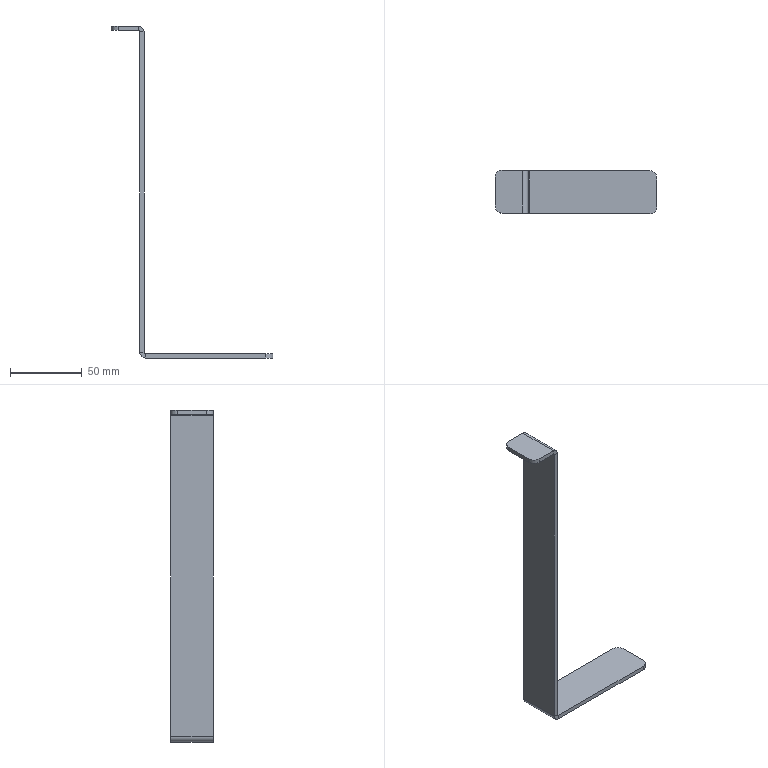Part | SolidWorks | features BreakCorner 1, FlatPattern 1, SMBaseFlange 1, SheetMetal 1 | 1 solid | 26 faces | box 113 x 30 x 232 mm | volume 30522 mm3 | plane 18 | cylinder 8 | commonest cylinder face diameters 10 x4 2 x2 8 x2
STEP:
#1=CARTESIAN_POINT('',(20.,15.,-1.));
#2=VERTEX_POINT('',#1);
#3=CARTESIAN_POINT('',(23.,15.,-1.));
#4=VERTEX_POINT('',#3);
#5=CARTESIAN_POINT('',(20.,15.,-1.));
#6=DIRECTION('',(1.,0.,0.));
#7=VECTOR('',#6,1000.);
#8=LINE('',#5,#7);
#9=EDGE_CURVE('',#2,#4,#8,.T.);
#10=ORIENTED_EDGE('',*,*,#9,.F.);
#11=CARTESIAN_POINT('',(19.,15.,0.));
#12=VERTEX_POINT('',#11);
#13=CARTESIAN_POINT('',(19.,15.,-1.));
#14=DIRECTION('',(0.,1.,0.));
#15=DIRECTION('',(0.,0.,-1.));
#16=AXIS2_PLACEMENT_3D('',#13,#14,#15);
#17=CIRCLE('',#16,1.);
#18=EDGE_CURVE('',#12,#2,#17,.T.);
#19=ORIENTED_EDGE('',*,*,#18,.F.);
#20=CARTESIAN_POINT('',(19.,15.,3.));
#21=VERTEX_POINT('',#20);
#22=CARTESIAN_POINT('',(19.,15.,3.));
#23=DIRECTION('',(0.,0.,-1.));
#24=VECTOR('',#23,1000.);
#25=LINE('',#22,#24);
#26=EDGE_CURVE('',#21,#12,#25,.T.);
#27=ORIENTED_EDGE('',*,*,#26,.F.);
#28=CARTESIAN_POINT('',(19.,15.,-1.));
#29=DIRECTION('',(0.,1.,0.));
#30=DIRECTION('',(1.,0.,0.));
#31=AXIS2_PLACEMENT_3D('',#28,#29,#30);
#32=CIRCLE('',#31,4.);
#33=EDGE_CURVE('',#21,#4,#32,.T.);
#34=ORIENTED_EDGE('',*,*,#33,.T.);
#35=EDGE_LOOP('',(#10,#19,#27,#34));
#36=FACE_OUTER_BOUND('',#35,.T.);
#37=CARTESIAN_POINT('',(20.,15.,-1.));
#38=DIRECTION('',(0.,1.,0.));
#39=DIRECTION('',(0.,0.,1.));
#40=AXIS2_PLACEMENT_3D('',#37,#38,#39);
#41=PLANE('',#40);
#42=ADVANCED_FACE('',(#36),#41,.T.);
#43=CARTESIAN_POINT('',(20.,15.,-225.));
#44=VERTEX_POINT('',#43);
#45=CARTESIAN_POINT('',(20.,15.,0.));
#46=DIRECTION('',(0.,0.,-1.));
#47=VECTOR('',#46,1000.);
#48=LINE('',#45,#47);
#49=EDGE_CURVE('',#2,#44,#48,.T.);
#50=ORIENTED_EDGE('',*,*,#49,.F.);
#51=ORIENTED_EDGE('',*,*,#9,.T.);
#52=CARTESIAN_POINT('',(23.,15.,-225.));
#53=VERTEX_POINT('',#52);
#54=CARTESIAN_POINT('',(23.,15.,0.));
#55=DIRECTION('',(0.,0.,-1.));
#56=VECTOR('',#55,1000.);
#57=LINE('',#54,#56);
#58=EDGE_CURVE('',#4,#53,#57,.T.);
#59=ORIENTED_EDGE('',*,*,#58,.T.);
#60=CARTESIAN_POINT('',(23.,15.,-225.));
#61=DIRECTION('',(-1.,0.,0.));
#62=VECTOR('',#61,1000.);
#63=LINE('',#60,#62);
#64=EDGE_CURVE('',#53,#44,#63,.T.);
#65=ORIENTED_EDGE('',*,*,#64,.T.);
#66=EDGE_LOOP('',(#50,#51,#59,#65));
#67=FACE_OUTER_BOUND('',#66,.T.);
#68=CARTESIAN_POINT('',(19.,15.,3.));
#69=DIRECTION('',(0.,1.,0.));
#70=DIRECTION('',(0.,0.,1.));
#71=AXIS2_PLACEMENT_3D('',#68,#69,#70);
#72=PLANE('',#71);
#73=ADVANCED_FACE('',(#67),#72,.T.);
#74=CARTESIAN_POINT('',(19.,-15.,0.));
#75=VERTEX_POINT('',#74);
#76=CARTESIAN_POINT('',(19.,-15.,3.));
#77=VERTEX_POINT('',#76);
#78=CARTESIAN_POINT('',(19.,-15.,0.));
#79=DIRECTION('',(0.,0.,1.));
#80=VECTOR('',#79,1000.);
#81=LINE('',#78,#80);
#82=EDGE_CURVE('',#75,#77,#81,.T.);
#83=ORIENTED_EDGE('',*,*,#82,.F.);
#84=CARTESIAN_POINT('',(20.,-15.,-1.));
#85=VERTEX_POINT('',#84);
#86=CARTESIAN_POINT('',(19.,-15.,-1.));
#87=DIRECTION('',(0.,1.,0.));
#88=DIRECTION('',(0.,0.,-1.));
#89=AXIS2_PLACEMENT_3D('',#86,#87,#88);
#90=CIRCLE('',#89,1.);
#91=EDGE_CURVE('',#75,#85,#90,.T.);
#92=ORIENTED_EDGE('',*,*,#91,.T.);
#93=CARTESIAN_POINT('',(23.,-15.,-1.));
#94=VERTEX_POINT('',#93);
#95=CARTESIAN_POINT('',(23.,-15.,-1.));
#96=DIRECTION('',(-1.,0.,0.));
#97=VECTOR('',#96,1000.);
#98=LINE('',#95,#97);
#99=EDGE_CURVE('',#94,#85,#98,.T.);
#100=ORIENTED_EDGE('',*,*,#99,.F.);
#101=CARTESIAN_POINT('',(19.,-15.,-1.));
#102=DIRECTION('',(0.,1.,0.));
#103=DIRECTION('',(1.,0.,0.));
#104=AXIS2_PLACEMENT_3D('',#101,#102,#103);
#105=CIRCLE('',#104,4.);
#106=EDGE_CURVE('',#77,#94,#105,.T.);
#107=ORIENTED_EDGE('',*,*,#106,.F.);
#108=EDGE_LOOP('',(#83,#92,#100,#107));
#109=FACE_OUTER_BOUND('',#108,.T.);
#110=CARTESIAN_POINT('',(19.,-15.,0.));
#111=DIRECTION('',(0.,-1.,0.));
#112=DIRECTION('',(0.,0.,-1.));
#113=AXIS2_PLACEMENT_3D('',#110,#111,#112);
#114=PLANE('',#113);
#115=ADVANCED_FACE('',(#109),#114,.T.);
#116=CARTESIAN_POINT('',(5.,-15.,3.));
#117=VERTEX_POINT('',#116);
#118=CARTESIAN_POINT('',(0.,-15.,3.));
#119=DIRECTION('',(1.,0.,0.));
#120=VECTOR('',#119,1000.);
#121=LINE('',#118,#120);
#122=EDGE_CURVE('',#117,#77,#121,.T.);
#123=ORIENTED_EDGE('',*,*,#122,.F.);
#124=CARTESIAN_POINT('',(5.,-15.,0.));
#125=VERTEX_POINT('',#124);
#126=CARTESIAN_POINT('',(5.,-15.,-1.));
#127=DIRECTION('',(0.,0.,-1.));
#128=VECTOR('',#127,1000.);
#129=LINE('',#126,#128);
#130=EDGE_CURVE('',#117,#125,#129,.T.);
#131=ORIENTED_EDGE('',*,*,#130,.T.);
#132=CARTESIAN_POINT('',(0.,-15.,0.));
#133=DIRECTION('',(1.,0.,0.));
#134=VECTOR('',#133,1000.);
#135=LINE('',#132,#134);
#136=EDGE_CURVE('',#125,#75,#135,.T.);
#137=ORIENTED_EDGE('',*,*,#136,.T.);
#138=ORIENTED_EDGE('',*,*,#82,.T.);
#139=EDGE_LOOP('',(#123,#131,#137,#138));
#140=FACE_OUTER_BOUND('',#139,.T.);
#141=CARTESIAN_POINT('',(23.,-15.,-1.));
#142=DIRECTION('',(0.,-1.,0.));
#143=DIRECTION('',(0.,0.,-1.));
#144=AXIS2_PLACEMENT_3D('',#141,#142,#143);
#145=PLANE('',#144);
#146=ADVANCED_FACE('',(#140),#145,.T.);
#147=CARTESIAN_POINT('',(24.,15.,-229.));
#148=VERTEX_POINT('',#147);
#149=CARTESIAN_POINT('',(24.,15.,-226.));
#150=VERTEX_POINT('',#149);
#151=CARTESIAN_POINT('',(24.,15.,-229.));
#152=DIRECTION('',(0.,0.,1.));
#153=VECTOR('',#152,1000.);
#154=LINE('',#151,#153);
#155=EDGE_CURVE('',#148,#150,#154,.T.);
#156=ORIENTED_EDGE('',*,*,#155,.F.);
#157=CARTESIAN_POINT('',(24.,15.,-225.));
#158=DIRECTION('',(0.,-1.,0.));
#159=DIRECTION('',(0.,0.,1.));
#160=AXIS2_PLACEMENT_3D('',#157,#158,#159);
#161=CIRCLE('',#160,4.);
#162=EDGE_CURVE('',#44,#148,#161,.T.);
#163=ORIENTED_EDGE('',*,*,#162,.F.);
#164=ORIENTED_EDGE('',*,*,#64,.F.);
#165=CARTESIAN_POINT('',(24.,15.,-225.));
#166=DIRECTION('',(0.,-1.,0.));
#167=DIRECTION('',(1.,0.,0.));
#168=AXIS2_PLACEMENT_3D('',#165,#166,#167);
#169=CIRCLE('',#168,1.);
#170=EDGE_CURVE('',#53,#150,#169,.T.);
#171=ORIENTED_EDGE('',*,*,#170,.T.);
#172=EDGE_LOOP('',(#156,#163,#164,#171));
#173=FACE_OUTER_BOUND('',#172,.T.);
#174=CARTESIAN_POINT('',(24.,15.,-229.));
#175=DIRECTION('',(0.,1.,0.));
#176=DIRECTION('',(0.,0.,1.));
#177=AXIS2_PLACEMENT_3D('',#174,#175,#176);
#178=PLANE('',#177);
#179=ADVANCED_FACE('',(#173),#178,.T.);
#180=CARTESIAN_POINT('',(108.,15.,-226.));
#181=VERTEX_POINT('',#180);
#182=CARTESIAN_POINT('',(20.,15.,-226.));
#183=DIRECTION('',(1.,0.,0.));
#184=VECTOR('',#183,1000.);
#185=LINE('',#182,#184);
#186=EDGE_CURVE('',#150,#181,#185,.T.);
#187=ORIENTED_EDGE('',*,*,#186,.T.);
#188=CARTESIAN_POINT('',(108.,15.,-229.));
#189=VERTEX_POINT('',#188);
#190=CARTESIAN_POINT('',(108.,15.,-225.));
#191=DIRECTION('',(0.,0.,-1.));
#192=VECTOR('',#191,1000.);
#193=LINE('',#190,#192);
#194=EDGE_CURVE('',#181,#189,#193,.T.);
#195=ORIENTED_EDGE('',*,*,#194,.T.);
#196=CARTESIAN_POINT('',(20.,15.,-229.));
#197=DIRECTION('',(1.,0.,0.));
#198=VECTOR('',#197,1000.);
#199=LINE('',#196,#198);
#200=EDGE_CURVE('',#148,#189,#199,.T.);
#201=ORIENTED_EDGE('',*,*,#200,.F.);
#202=ORIENTED_EDGE('',*,*,#155,.T.);
#203=EDGE_LOOP('',(#187,#195,#201,#202));
#204=FACE_OUTER_BOUND('',#203,.T.);
#205=CARTESIAN_POINT('',(23.,15.,-225.));
#206=DIRECTION('',(0.,1.,0.));
#207=DIRECTION('',(0.,0.,1.));
#208=AXIS2_PLACEMENT_3D('',#205,#206,#207);
#209=PLANE('',#208);
#210=ADVANCED_FACE('',(#204),#209,.T.);
#211=CARTESIAN_POINT('',(20.,-15.,-225.));
#212=VERTEX_POINT('',#211);
#213=CARTESIAN_POINT('',(23.,-15.,-225.));
#214=VERTEX_POINT('',#213);
#215=CARTESIAN_POINT('',(20.,-15.,-225.));
#216=DIRECTION('',(1.,0.,0.));
#217=VECTOR('',#216,1000.);
#218=LINE('',#215,#217);
#219=EDGE_CURVE('',#212,#214,#218,.T.);
#220=ORIENTED_EDGE('',*,*,#219,.F.);
#221=CARTESIAN_POINT('',(24.,-15.,-229.));
#222=VERTEX_POINT('',#221);
#223=CARTESIAN_POINT('',(24.,-15.,-225.));
#224=DIRECTION('',(0.,-1.,0.));
#225=DIRECTION('',(0.,0.,1.));
#226=AXIS2_PLACEMENT_3D('',#223,#224,#225);
#227=CIRCLE('',#226,4.);
#228=EDGE_CURVE('',#212,#222,#227,.T.);
#229=ORIENTED_EDGE('',*,*,#228,.T.);
#230=CARTESIAN_POINT('',(24.,-15.,-226.));
#231=VERTEX_POINT('',#230);
#232=CARTESIAN_POINT('',(24.,-15.,-226.));
#233=DIRECTION('',(0.,0.,-1.));
#234=VECTOR('',#233,1000.);
#235=LINE('',#232,#234);
#236=EDGE_CURVE('',#231,#222,#235,.T.);
#237=ORIENTED_EDGE('',*,*,#236,.F.);
#238=CARTESIAN_POINT('',(24.,-15.,-225.));
#239=DIRECTION('',(0.,-1.,0.));
#240=DIRECTION('',(1.,0.,0.));
#241=AXIS2_PLACEMENT_3D('',#238,#239,#240);
#242=CIRCLE('',#241,1.);
#243=EDGE_CURVE('',#214,#231,#242,.T.);
#244=ORIENTED_EDGE('',*,*,#243,.F.);
#245=EDGE_LOOP('',(#220,#229,#237,#244));
#246=FACE_OUTER_BOUND('',#245,.T.);
#247=CARTESIAN_POINT('',(20.,-15.,-225.));
#248=DIRECTION('',(0.,-1.,0.));
#249=DIRECTION('',(0.,0.,-1.));
#250=AXIS2_PLACEMENT_3D('',#247,#248,#249);
#251=PLANE('',#250);
#252=ADVANCED_FACE('',(#246),#251,.T.);
#253=CARTESIAN_POINT('',(20.,-15.,0.));
#254=DIRECTION('',(0.,0.,-1.));
#255=VECTOR('',#254,1000.);
#256=LINE('',#253,#255);
#257=EDGE_CURVE('',#85,#212,#256,.T.);
#258=ORIENTED_EDGE('',*,*,#257,.T.);
#259=ORIENTED_EDGE('',*,*,#219,.T.);
#260=CARTESIAN_POINT('',(23.,-15.,0.));
#261=DIRECTION('',(0.,0.,-1.));
#262=VECTOR('',#261,1000.);
#263=LINE('',#260,#262);
#264=EDGE_CURVE('',#94,#214,#263,.T.);
#265=ORIENTED_EDGE('',*,*,#264,.F.);
#266=ORIENTED_EDGE('',*,*,#99,.T.);
#267=EDGE_LOOP('',(#258,#259,#265,#266));
#268=FACE_OUTER_BOUND('',#267,.T.);
#269=CARTESIAN_POINT('',(24.,-15.,-226.));
#270=DIRECTION('',(0.,-1.,0.));
#271=DIRECTION('',(0.,0.,-1.));
#272=AXIS2_PLACEMENT_3D('',#269,#270,#271);
#273=PLANE('',#272);
#274=ADVANCED_FACE('',(#268),#273,.T.);
#275=CARTESIAN_POINT('',(113.,10.,-226.));
#276=VERTEX_POINT('',#275);
#277=CARTESIAN_POINT('',(113.,-10.,-226.));
#278=VERTEX_POINT('',#277);
#279=CARTESIAN_POINT('',(113.,15.,-226.));
#280=DIRECTION('',(0.,-1.,0.));
#281=VECTOR('',#280,1000.);
#282=LINE('',#279,#281);
#283=EDGE_CURVE('',#276,#278,#282,.T.);
#284=ORIENTED_EDGE('',*,*,#283,.F.);
#285=CARTESIAN_POINT('',(108.,10.,-226.));
#286=DIRECTION('',(0.,0.,1.));
#287=DIRECTION('',(-1.,0.,0.));
#288=AXIS2_PLACEMENT_3D('',#285,#286,#287);
#289=CIRCLE('',#288,5.);
#290=EDGE_CURVE('',#276,#181,#289,.T.);
#291=ORIENTED_EDGE('',*,*,#290,.T.);
#292=ORIENTED_EDGE('',*,*,#186,.F.);
#293=CARTESIAN_POINT('',(24.,15.,-226.));
#294=DIRECTION('',(0.,-1.,0.));
#295=VECTOR('',#294,1000.);
#296=LINE('',#293,#295);
#297=EDGE_CURVE('',#150,#231,#296,.T.);
#298=ORIENTED_EDGE('',*,*,#297,.T.);
#299=CARTESIAN_POINT('',(108.,-15.,-226.));
#300=VERTEX_POINT('',#299);
#301=CARTESIAN_POINT('',(20.,-15.,-226.));
#302=DIRECTION('',(1.,0.,0.));
#303=VECTOR('',#302,1000.);
#304=LINE('',#301,#303);
#305=EDGE_CURVE('',#231,#300,#304,.T.);
#306=ORIENTED_EDGE('',*,*,#305,.T.);
#307=CARTESIAN_POINT('',(108.,-10.,-226.));
#308=DIRECTION('',(0.,0.,1.));
#309=DIRECTION('',(-1.,0.,0.));
#310=AXIS2_PLACEMENT_3D('',#307,#308,#309);
#311=CIRCLE('',#310,5.);
#312=EDGE_CURVE('',#300,#278,#311,.T.);
#313=ORIENTED_EDGE('',*,*,#312,.T.);
#314=EDGE_LOOP('',(#284,#291,#292,#298,#306,#313));
#315=FACE_OUTER_BOUND('',#314,.T.);
#316=CARTESIAN_POINT('',(20.,15.,-226.));
#317=DIRECTION('',(0.,0.,-1.));
#318=DIRECTION('',(-1.,0.,0.));
#319=AXIS2_PLACEMENT_3D('',#316,#317,#318);
#320=PLANE('',#319);
#321=ADVANCED_FACE('',(#315),#320,.F.);
#322=CARTESIAN_POINT('',(113.,10.,-229.));
#323=VERTEX_POINT('',#322);
#324=CARTESIAN_POINT('',(113.,-10.,-229.));
#325=VERTEX_POINT('',#324);
#326=CARTESIAN_POINT('',(113.,15.,-229.));
#327=DIRECTION('',(0.,-1.,0.));
#328=VECTOR('',#327,1000.);
#329=LINE('',#326,#328);
#330=EDGE_CURVE('',#323,#325,#329,.T.);
#331=ORIENTED_EDGE('',*,*,#330,.F.);
#332=CARTESIAN_POINT('',(113.,10.,-229.));
#333=DIRECTION('',(0.,0.,1.));
#334=VECTOR('',#333,1000.);
#335=LINE('',#332,#334);
#336=EDGE_CURVE('',#323,#276,#335,.T.);
#337=ORIENTED_EDGE('',*,*,#336,.T.);
#338=ORIENTED_EDGE('',*,*,#283,.T.);
#339=CARTESIAN_POINT('',(113.,-10.,-229.));
#340=DIRECTION('',(0.,0.,-1.));
#341=VECTOR('',#340,1000.);
#342=LINE('',#339,#341);
#343=EDGE_CURVE('',#278,#325,#342,.T.);
#344=ORIENTED_EDGE('',*,*,#343,.T.);
#345=EDGE_LOOP('',(#331,#337,#338,#344));
#346=FACE_OUTER_BOUND('',#345,.T.);
#347=CARTESIAN_POINT('',(113.,15.,-229.));
#348=DIRECTION('',(1.,0.,0.));
#349=DIRECTION('',(0.,0.,-1.));
#350=AXIS2_PLACEMENT_3D('',#347,#348,#349);
#351=PLANE('',#350);
#352=ADVANCED_FACE('',(#346),#351,.T.);
#353=ORIENTED_EDGE('',*,*,#200,.T.);
#354=CARTESIAN_POINT('',(108.,10.,-229.));
#355=DIRECTION('',(0.,0.,-1.));
#356=DIRECTION('',(-1.,0.,0.));
#357=AXIS2_PLACEMENT_3D('',#354,#355,#356);
#358=CIRCLE('',#357,5.);
#359=EDGE_CURVE('',#189,#323,#358,.T.);
#360=ORIENTED_EDGE('',*,*,#359,.T.);
#361=ORIENTED_EDGE('',*,*,#330,.T.);
#362=CARTESIAN_POINT('',(108.,-15.,-229.));
#363=VERTEX_POINT('',#362);
#364=CARTESIAN_POINT('',(108.,-10.,-229.));
#365=DIRECTION('',(0.,0.,-1.));
#366=DIRECTION('',(-1.,0.,0.));
#367=AXIS2_PLACEMENT_3D('',#364,#365,#366);
#368=CIRCLE('',#367,5.);
#369=EDGE_CURVE('',#325,#363,#368,.T.);
#370=ORIENTED_EDGE('',*,*,#369,.T.);
#371=CARTESIAN_POINT('',(20.,-15.,-229.));
#372=DIRECTION('',(1.,0.,0.));
#373=VECTOR('',#372,1000.);
#374=LINE('',#371,#373);
#375=EDGE_CURVE('',#222,#363,#374,.T.);
#376=ORIENTED_EDGE('',*,*,#375,.F.);
#377=CARTESIAN_POINT('',(24.,15.,-229.));
#378=DIRECTION('',(0.,-1.,0.));
#379=VECTOR('',#378,1000.);
#380=LINE('',#377,#379);
#381=EDGE_CURVE('',#148,#222,#380,.T.);
#382=ORIENTED_EDGE('',*,*,#381,.F.);
#383=EDGE_LOOP('',(#353,#360,#361,#370,#376,#382));
#384=FACE_OUTER_BOUND('',#383,.T.);
#385=CARTESIAN_POINT('',(20.,15.,-229.));
#386=DIRECTION('',(0.,0.,-1.));
#387=DIRECTION('',(-1.,0.,0.));
#388=AXIS2_PLACEMENT_3D('',#385,#386,#387);
#389=PLANE('',#388);
#390=ADVANCED_FACE('',(#384),#389,.T.);
#391=ORIENTED_EDGE('',*,*,#228,.F.);
#392=CARTESIAN_POINT('',(20.,15.,-225.));
#393=DIRECTION('',(0.,-1.,0.));
#394=VECTOR('',#393,1000.);
#395=LINE('',#392,#394);
#396=EDGE_CURVE('',#44,#212,#395,.T.);
#397=ORIENTED_EDGE('',*,*,#396,.F.);
#398=ORIENTED_EDGE('',*,*,#162,.T.);
#399=ORIENTED_EDGE('',*,*,#381,.T.);
#400=EDGE_LOOP('',(#391,#397,#398,#399));
#401=FACE_OUTER_BOUND('',#400,.T.);
#402=CARTESIAN_POINT('',(24.,15.,-225.));
#403=DIRECTION('',(0.,-1.,0.));
#404=DIRECTION('',(0.,0.,-1.));
#405=AXIS2_PLACEMENT_3D('',#402,#403,#404);
#406=CYLINDRICAL_SURFACE('',#405,4.);
#407=ADVANCED_FACE('',(#401),#406,.T.);
#408=ORIENTED_EDGE('',*,*,#257,.F.);
#409=CARTESIAN_POINT('',(20.,15.,-1.));
#410=DIRECTION('',(0.,-1.,0.));
#411=VECTOR('',#410,1000.);
#412=LINE('',#409,#411);
#413=EDGE_CURVE('',#2,#85,#412,.T.);
#414=ORIENTED_EDGE('',*,*,#413,.F.);
#415=ORIENTED_EDGE('',*,*,#49,.T.);
#416=ORIENTED_EDGE('',*,*,#396,.T.);
#417=EDGE_LOOP('',(#408,#414,#415,#416));
#418=FACE_OUTER_BOUND('',#417,.T.);
#419=CARTESIAN_POINT('',(20.,15.,0.));
#420=DIRECTION('',(-1.,0.,0.));
#421=DIRECTION('',(0.,0.,1.));
#422=AXIS2_PLACEMENT_3D('',#419,#420,#421);
#423=PLANE('',#422);
#424=ADVANCED_FACE('',(#418),#423,.T.);
#425=ORIENTED_EDGE('',*,*,#91,.F.);
#426=CARTESIAN_POINT('',(19.,15.,0.));
#427=DIRECTION('',(0.,-1.,0.));
#428=VECTOR('',#427,1000.);
#429=LINE('',#426,#428);
#430=EDGE_CURVE('',#12,#75,#429,.T.);
#431=ORIENTED_EDGE('',*,*,#430,.F.);
#432=ORIENTED_EDGE('',*,*,#18,.T.);
#433=ORIENTED_EDGE('',*,*,#413,.T.);
#434=EDGE_LOOP('',(#425,#431,#432,#433));
#435=FACE_OUTER_BOUND('',#434,.T.);
#436=CARTESIAN_POINT('',(19.,15.,-1.));
#437=DIRECTION('',(0.,-1.,0.));
#438=DIRECTION('',(0.,0.,-1.));
#439=AXIS2_PLACEMENT_3D('',#436,#437,#438);
#440=CYLINDRICAL_SURFACE('',#439,1.);
#441=ADVANCED_FACE('',(#435),#440,.F.);
#442=CARTESIAN_POINT('',(0.,10.,0.));
#443=VERTEX_POINT('',#442);
#444=CARTESIAN_POINT('',(0.,-10.,0.));
#445=VERTEX_POINT('',#444);
#446=CARTESIAN_POINT('',(0.,15.,0.));
#447=DIRECTION('',(0.,-1.,0.));
#448=VECTOR('',#447,1000.);
#449=LINE('',#446,#448);
#450=EDGE_CURVE('',#443,#445,#449,.T.);
#451=ORIENTED_EDGE('',*,*,#450,.F.);
#452=CARTESIAN_POINT('',(5.,15.,0.));
#453=VERTEX_POINT('',#452);
#454=CARTESIAN_POINT('',(5.,10.,0.));
#455=DIRECTION('',(0.,0.,-1.));
#456=DIRECTION('',(-1.,0.,0.));
#457=AXIS2_PLACEMENT_3D('',#454,#455,#456);
#458=CIRCLE('',#457,5.);
#459=EDGE_CURVE('',#443,#453,#458,.T.);
#460=ORIENTED_EDGE('',*,*,#459,.T.);
#461=CARTESIAN_POINT('',(0.,15.,0.));
#462=DIRECTION('',(1.,0.,0.));
#463=VECTOR('',#462,1000.);
#464=LINE('',#461,#463);
#465=EDGE_CURVE('',#453,#12,#464,.T.);
#466=ORIENTED_EDGE('',*,*,#465,.T.);
#467=ORIENTED_EDGE('',*,*,#430,.T.);
#468=ORIENTED_EDGE('',*,*,#136,.F.);
#469=CARTESIAN_POINT('',(5.,-10.,0.));
#470=DIRECTION('',(0.,0.,-1.));
#471=DIRECTION('',(-1.,0.,0.));
#472=AXIS2_PLACEMENT_3D('',#469,#470,#471);
#473=CIRCLE('',#472,5.);
#474=EDGE_CURVE('',#125,#445,#473,.T.);
#475=ORIENTED_EDGE('',*,*,#474,.T.);
#476=EDGE_LOOP('',(#451,#460,#466,#467,#468,#475));
#477=FACE_OUTER_BOUND('',#476,.T.);
#478=CARTESIAN_POINT('',(0.,15.,0.));
#479=DIRECTION('',(0.,0.,-1.));
#480=DIRECTION('',(-1.,0.,0.));
#481=AXIS2_PLACEMENT_3D('',#478,#479,#480);
#482=PLANE('',#481);
#483=ADVANCED_FACE('',(#477),#482,.T.);
#484=CARTESIAN_POINT('',(0.,10.,3.));
#485=VERTEX_POINT('',#484);
#486=CARTESIAN_POINT('',(0.,-10.,3.));
#487=VERTEX_POINT('',#486);
#488=CARTESIAN_POINT('',(0.,15.,3.));
#489=DIRECTION('',(0.,-1.,0.));
#490=VECTOR('',#489,1000.);
#491=LINE('',#488,#490);
#492=EDGE_CURVE('',#485,#487,#491,.T.);
#493=ORIENTED_EDGE('',*,*,#492,.F.);
#494=CARTESIAN_POINT('',(0.,10.,3.));
#495=DIRECTION('',(0.,0.,-1.));
#496=VECTOR('',#495,1000.);
#497=LINE('',#494,#496);
#498=EDGE_CURVE('',#485,#443,#497,.T.);
#499=ORIENTED_EDGE('',*,*,#498,.T.);
#500=ORIENTED_EDGE('',*,*,#450,.T.);
#501=CARTESIAN_POINT('',(0.,-10.,3.));
#502=DIRECTION('',(0.,0.,1.));
#503=VECTOR('',#502,1000.);
#504=LINE('',#501,#503);
#505=EDGE_CURVE('',#445,#487,#504,.T.);
#506=ORIENTED_EDGE('',*,*,#505,.T.);
#507=EDGE_LOOP('',(#493,#499,#500,#506));
#508=FACE_OUTER_BOUND('',#507,.T.);
#509=CARTESIAN_POINT('',(0.,15.,3.));
#510=DIRECTION('',(-1.,0.,0.));
#511=DIRECTION('',(0.,0.,1.));
#512=AXIS2_PLACEMENT_3D('',#509,#510,#511);
#513=PLANE('',#512);
#514=ADVANCED_FACE('',(#508),#513,.T.);
#515=CARTESIAN_POINT('',(5.,15.,3.));
#516=VERTEX_POINT('',#515);
#517=CARTESIAN_POINT('',(0.,15.,3.));
#518=DIRECTION('',(1.,0.,0.));
#519=VECTOR('',#518,1000.);
#520=LINE('',#517,#519);
#521=EDGE_CURVE('',#516,#21,#520,.T.);
#522=ORIENTED_EDGE('',*,*,#521,.F.);
#523=CARTESIAN_POINT('',(5.,10.,3.));
#524=DIRECTION('',(0.,0.,1.));
#525=DIRECTION('',(-1.,0.,0.));
#526=AXIS2_PLACEMENT_3D('',#523,#524,#525);
#527=CIRCLE('',#526,5.);
#528=EDGE_CURVE('',#516,#485,#527,.T.);
#529=ORIENTED_EDGE('',*,*,#528,.T.);
#530=ORIENTED_EDGE('',*,*,#492,.T.);
#531=CARTESIAN_POINT('',(5.,-10.,3.));
#532=DIRECTION('',(0.,0.,1.));
#533=DIRECTION('',(-1.,0.,0.));
#534=AXIS2_PLACEMENT_3D('',#531,#532,#533);
#535=CIRCLE('',#534,5.);
#536=EDGE_CURVE('',#487,#117,#535,.T.);
#537=ORIENTED_EDGE('',*,*,#536,.T.);
#538=ORIENTED_EDGE('',*,*,#122,.T.);
#539=CARTESIAN_POINT('',(19.,15.,3.));
#540=DIRECTION('',(0.,-1.,0.));
#541=VECTOR('',#540,1000.);
#542=LINE('',#539,#541);
#543=EDGE_CURVE('',#21,#77,#542,.T.);
#544=ORIENTED_EDGE('',*,*,#543,.F.);
#545=EDGE_LOOP('',(#522,#529,#530,#537,#538,#544));
#546=FACE_OUTER_BOUND('',#545,.T.);
#547=CARTESIAN_POINT('',(0.,15.,3.));
#548=DIRECTION('',(0.,0.,-1.));
#549=DIRECTION('',(-1.,0.,0.));
#550=AXIS2_PLACEMENT_3D('',#547,#548,#549);
#551=PLANE('',#550);
#552=ADVANCED_FACE('',(#546),#551,.F.);
#553=ORIENTED_EDGE('',*,*,#106,.T.);
#554=CARTESIAN_POINT('',(23.,15.,-1.));
#555=DIRECTION('',(0.,-1.,0.));
#556=VECTOR('',#555,1000.);
#557=LINE('',#554,#556);
#558=EDGE_CURVE('',#4,#94,#557,.T.);
#559=ORIENTED_EDGE('',*,*,#558,.F.);
#560=ORIENTED_EDGE('',*,*,#33,.F.);
#561=ORIENTED_EDGE('',*,*,#543,.T.);
#562=EDGE_LOOP('',(#553,#559,#560,#561));
#563=FACE_OUTER_BOUND('',#562,.T.);
#564=CARTESIAN_POINT('',(19.,15.,-1.));
#565=DIRECTION('',(0.,-1.,0.));
#566=DIRECTION('',(0.,0.,-1.));
#567=AXIS2_PLACEMENT_3D('',#564,#565,#566);
#568=CYLINDRICAL_SURFACE('',#567,4.);
#569=ADVANCED_FACE('',(#563),#568,.T.);
#570=ORIENTED_EDGE('',*,*,#264,.T.);
#571=CARTESIAN_POINT('',(23.,15.,-225.));
#572=DIRECTION('',(0.,-1.,0.));
#573=VECTOR('',#572,1000.);
#574=LINE('',#571,#573);
#575=EDGE_CURVE('',#53,#214,#574,.T.);
#576=ORIENTED_EDGE('',*,*,#575,.F.);
#577=ORIENTED_EDGE('',*,*,#58,.F.);
#578=ORIENTED_EDGE('',*,*,#558,.T.);
#579=EDGE_LOOP('',(#570,#576,#577,#578));
#580=FACE_OUTER_BOUND('',#579,.T.);
#581=CARTESIAN_POINT('',(23.,15.,0.));
#582=DIRECTION('',(-1.,0.,0.));
#583=DIRECTION('',(0.,0.,1.));
#584=AXIS2_PLACEMENT_3D('',#581,#582,#583);
#585=PLANE('',#584);
#586=ADVANCED_FACE('',(#580),#585,.F.);
#587=ORIENTED_EDGE('',*,*,#243,.T.);
#588=ORIENTED_EDGE('',*,*,#297,.F.);
#589=ORIENTED_EDGE('',*,*,#170,.F.);
#590=ORIENTED_EDGE('',*,*,#575,.T.);
#591=EDGE_LOOP('',(#587,#588,#589,#590));
#592=FACE_OUTER_BOUND('',#591,.T.);
#593=CARTESIAN_POINT('',(24.,15.,-225.));
#594=DIRECTION('',(0.,-1.,0.));
#595=DIRECTION('',(0.,0.,-1.));
#596=AXIS2_PLACEMENT_3D('',#593,#594,#595);
#597=CYLINDRICAL_SURFACE('',#596,1.);
#598=ADVANCED_FACE('',(#592),#597,.F.);
#599=ORIENTED_EDGE('',*,*,#465,.F.);
#600=CARTESIAN_POINT('',(5.,15.,-225.));
#601=DIRECTION('',(0.,0.,1.));
#602=VECTOR('',#601,1000.);
#603=LINE('',#600,#602);
#604=EDGE_CURVE('',#453,#516,#603,.T.);
#605=ORIENTED_EDGE('',*,*,#604,.T.);
#606=ORIENTED_EDGE('',*,*,#521,.T.);
#607=ORIENTED_EDGE('',*,*,#26,.T.);
#608=EDGE_LOOP('',(#599,#605,#606,#607));
#609=FACE_OUTER_BOUND('',#608,.T.);
#610=CARTESIAN_POINT('',(24.,15.,-225.));
#611=DIRECTION('',(0.,1.,0.));
#612=DIRECTION('',(1.,0.,0.));
#613=AXIS2_PLACEMENT_3D('',#610,#611,#612);
#614=PLANE('',#613);
#615=ADVANCED_FACE('',(#609),#614,.T.);
#616=ORIENTED_EDGE('',*,*,#375,.T.);
#617=CARTESIAN_POINT('',(108.,-15.,-226.));
#618=DIRECTION('',(0.,0.,1.));
#619=VECTOR('',#618,1000.);
#620=LINE('',#617,#619);
#621=EDGE_CURVE('',#363,#300,#620,.T.);
#622=ORIENTED_EDGE('',*,*,#621,.T.);
#623=ORIENTED_EDGE('',*,*,#305,.F.);
#624=ORIENTED_EDGE('',*,*,#236,.T.);
#625=EDGE_LOOP('',(#616,#622,#623,#624));
#626=FACE_OUTER_BOUND('',#625,.T.);
#627=CARTESIAN_POINT('',(24.,-15.,-225.));
#628=DIRECTION('',(0.,1.,0.));
#629=DIRECTION('',(1.,0.,0.));
#630=AXIS2_PLACEMENT_3D('',#627,#628,#629);
#631=PLANE('',#630);
#632=ADVANCED_FACE('',(#626),#631,.F.);
#633=ORIENTED_EDGE('',*,*,#528,.F.);
#634=ORIENTED_EDGE('',*,*,#604,.F.);
#635=ORIENTED_EDGE('',*,*,#459,.F.);
#636=ORIENTED_EDGE('',*,*,#498,.F.);
#637=EDGE_LOOP('',(#633,#634,#635,#636));
#638=FACE_OUTER_BOUND('',#637,.T.);
#639=CARTESIAN_POINT('',(5.,10.,3.));
#640=DIRECTION('',(0.,0.,-1.));
#641=DIRECTION('',(-1.,0.,0.));
#642=AXIS2_PLACEMENT_3D('',#639,#640,#641);
#643=CYLINDRICAL_SURFACE('',#642,5.);
#644=ADVANCED_FACE('',(#638),#643,.T.);
#645=ORIENTED_EDGE('',*,*,#536,.F.);
#646=ORIENTED_EDGE('',*,*,#505,.F.);
#647=ORIENTED_EDGE('',*,*,#474,.F.);
#648=ORIENTED_EDGE('',*,*,#130,.F.);
#649=EDGE_LOOP('',(#645,#646,#647,#648));
#650=FACE_OUTER_BOUND('',#649,.T.);
#651=CARTESIAN_POINT('',(5.,-10.,-1.));
#652=DIRECTION('',(0.,0.,-1.));
#653=DIRECTION('',(-1.,0.,0.));
#654=AXIS2_PLACEMENT_3D('',#651,#652,#653);
#655=CYLINDRICAL_SURFACE('',#654,5.);
#656=ADVANCED_FACE('',(#650),#655,.T.);
#657=ORIENTED_EDGE('',*,*,#359,.F.);
#658=ORIENTED_EDGE('',*,*,#194,.F.);
#659=ORIENTED_EDGE('',*,*,#290,.F.);
#660=ORIENTED_EDGE('',*,*,#336,.F.);
#661=EDGE_LOOP('',(#657,#658,#659,#660));
#662=FACE_OUTER_BOUND('',#661,.T.);
#663=CARTESIAN_POINT('',(108.,10.,-229.));
#664=DIRECTION('',(0.,0.,1.));
#665=DIRECTION('',(1.,0.,0.));
#666=AXIS2_PLACEMENT_3D('',#663,#664,#665);
#667=CYLINDRICAL_SURFACE('',#666,5.);
#668=ADVANCED_FACE('',(#662),#667,.T.);
#669=ORIENTED_EDGE('',*,*,#369,.F.);
#670=ORIENTED_EDGE('',*,*,#343,.F.);
#671=ORIENTED_EDGE('',*,*,#312,.F.);
#672=ORIENTED_EDGE('',*,*,#621,.F.);
#673=EDGE_LOOP('',(#669,#670,#671,#672));
#674=FACE_OUTER_BOUND('',#673,.T.);
#675=CARTESIAN_POINT('',(108.,-10.,-225.));
#676=DIRECTION('',(0.,0.,-1.));
#677=DIRECTION('',(-1.,0.,0.));
#678=AXIS2_PLACEMENT_3D('',#675,#676,#677);
#679=CYLINDRICAL_SURFACE('',#678,5.);
#680=ADVANCED_FACE('',(#674),#679,.T.);
#681=CLOSED_SHELL('',(#42,#73,#115,#146,#179,#210,#252,#274,#321,#352,#390,#407,#424,#441,#483,#514,#552,#569,#586,#598,#615,#632,#644,#656,#668,#680));
#682=MANIFOLD_SOLID_BREP('',#681);
#683=CARTESIAN_POINT('',(0.,0.,0.));
#684=DIRECTION('',(0.,0.,1.));
#685=DIRECTION('',(1.,0.,0.));
#686=AXIS2_PLACEMENT_3D('',#683,#684,#685);
#687=(LENGTH_UNIT()NAMED_UNIT(*)SI_UNIT(.MILLI.,.METRE.));
#688=UNCERTAINTY_MEASURE_WITH_UNIT(LENGTH_MEASURE(0.00001),#687,'','');
#689=(NAMED_UNIT(*)PLANE_ANGLE_UNIT()SI_UNIT($,.RADIAN.));
#690=(NAMED_UNIT(*)SI_UNIT($,.STERADIAN.)SOLID_ANGLE_UNIT());
#691=(GEOMETRIC_REPRESENTATION_CONTEXT(3)GLOBAL_UNCERTAINTY_ASSIGNED_CONTEXT((#688))GLOBAL_UNIT_ASSIGNED_CONTEXT((#687,#689,#690))REPRESENTATION_CONTEXT('',''));
#692=ADVANCED_BREP_SHAPE_REPRESENTATION('',(#682,#686),#691);